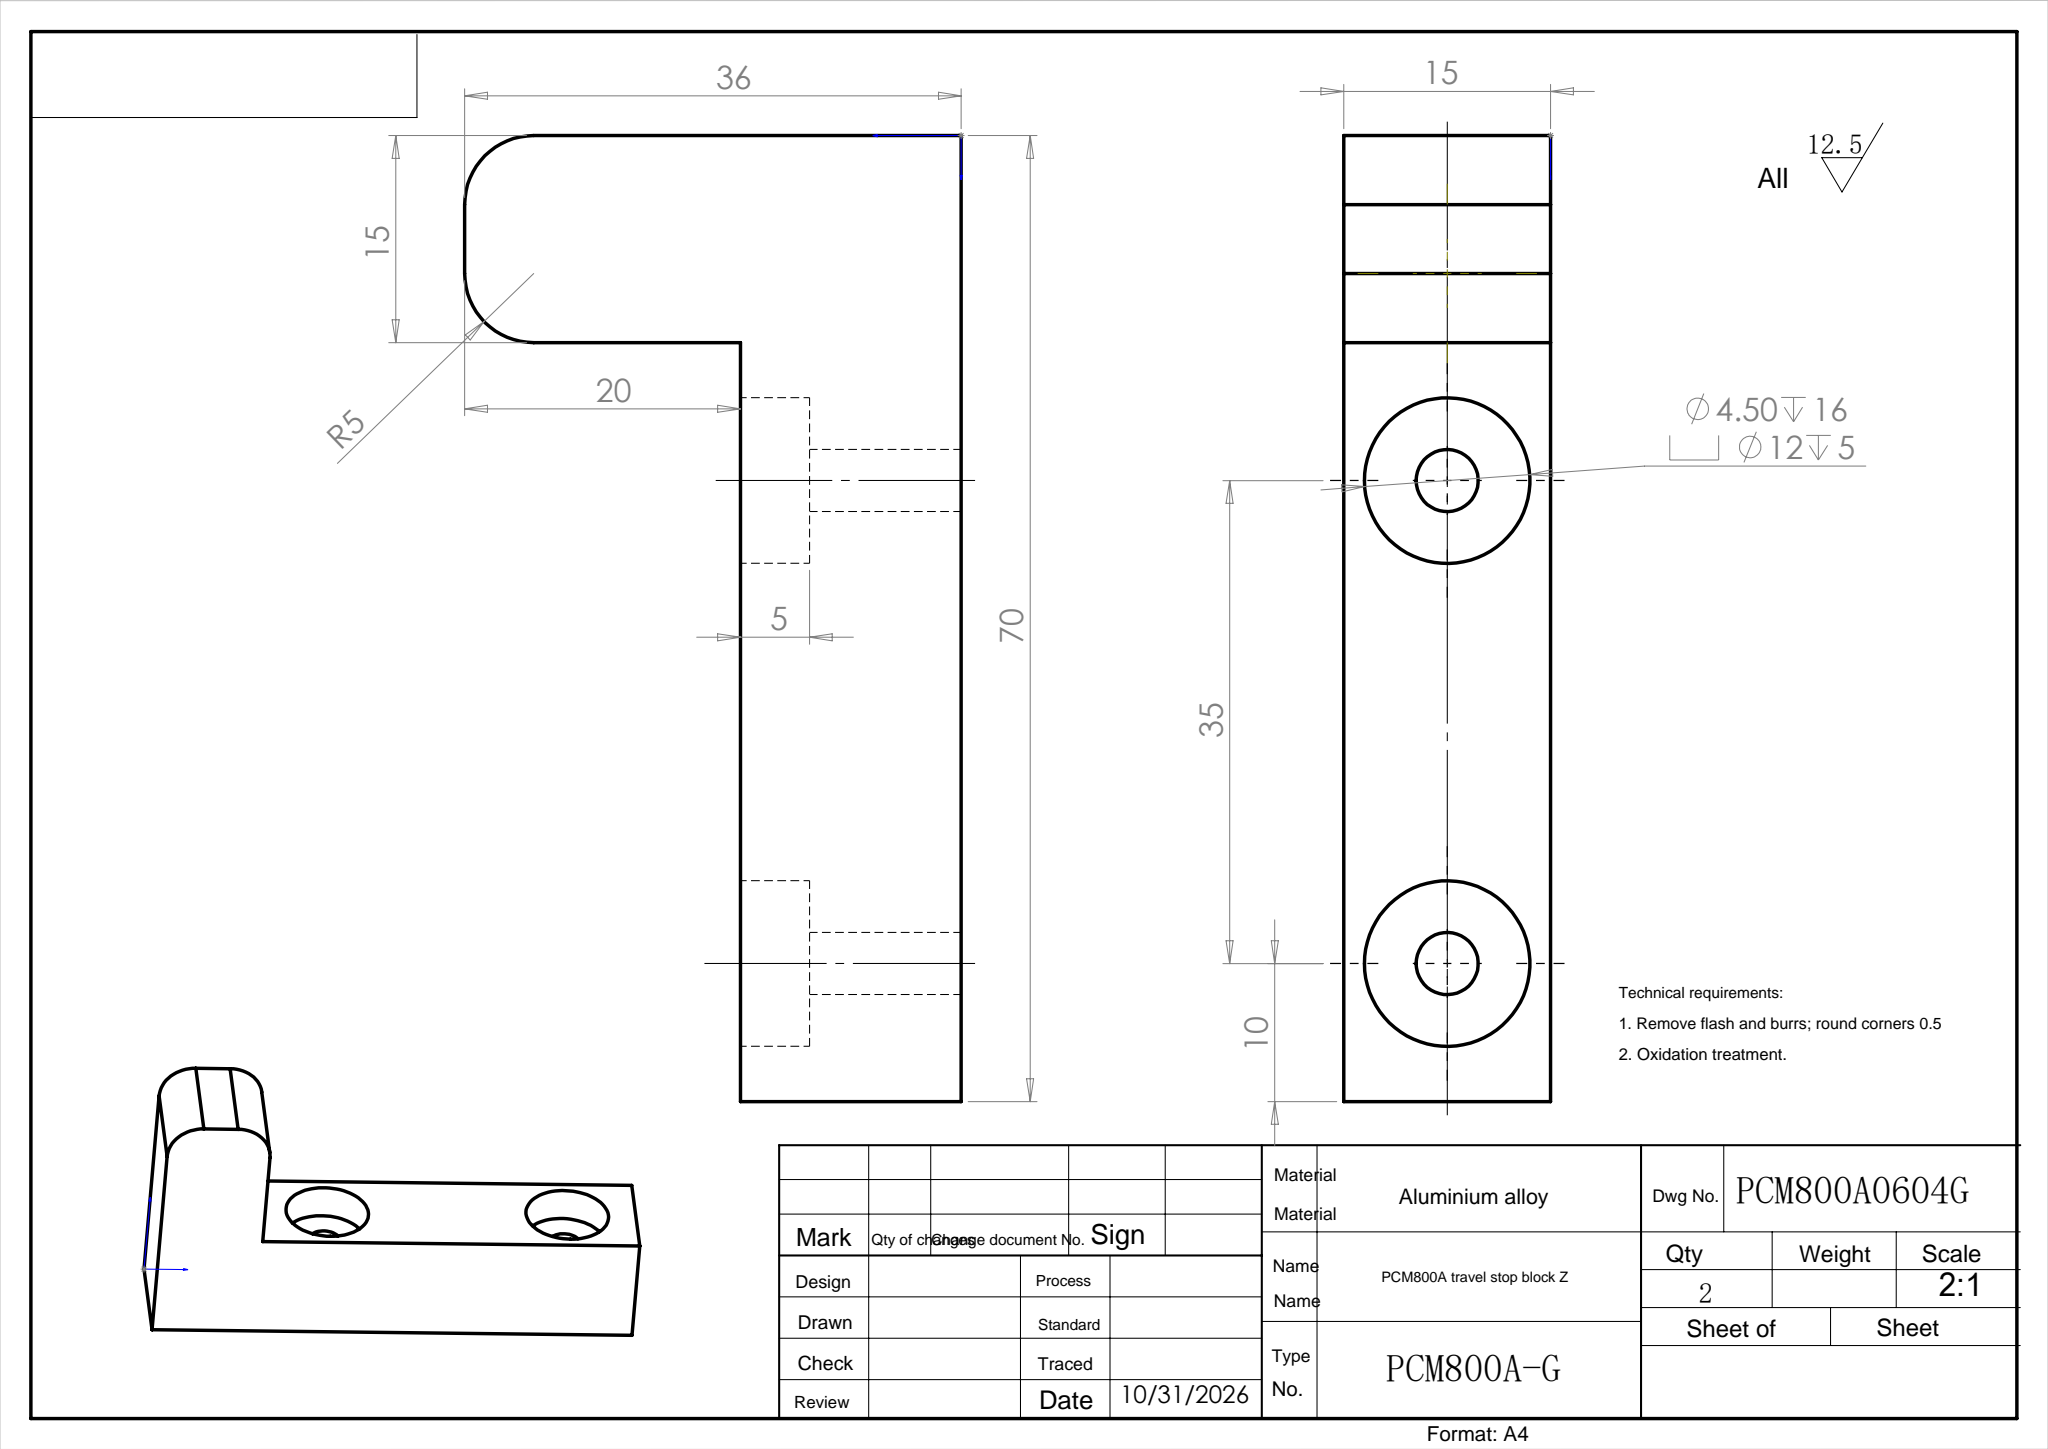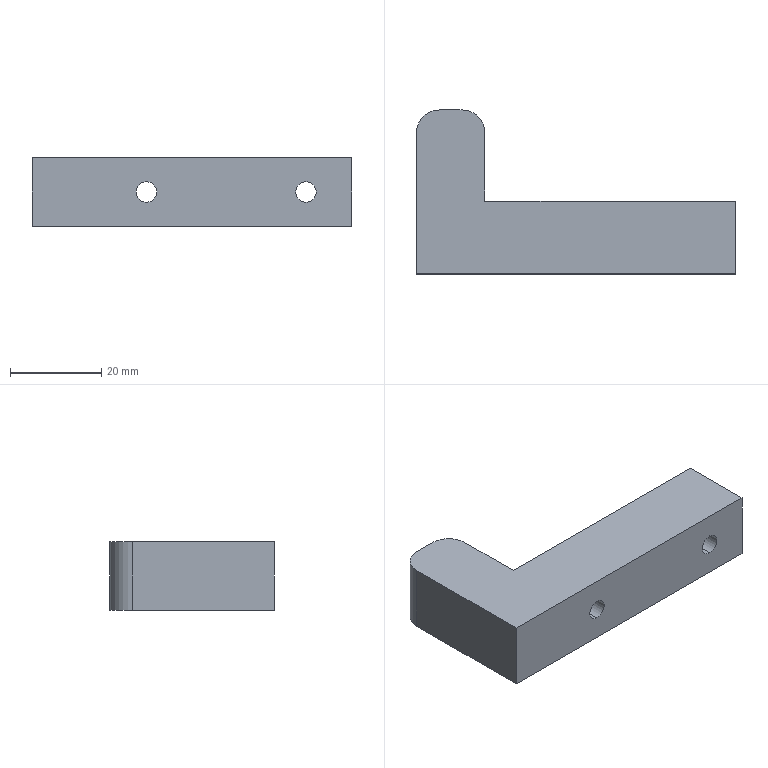Part | SolidWorks | features Extrusion 1, Fillet 1, HoleWzd 1 | 1 solid | 20 faces | box 70 x 36 x 15 mm | volume 19658 mm3 | cylinder 10 | plane 10 | commonest cylinder face diameters 4.5 x4 12 x4 10 x2
STEP:
#1=CARTESIAN_POINT('',(25.,11.,1.5));
#2=VERTEX_POINT('',#1);
#3=CARTESIAN_POINT('',(25.,11.,13.5));
#4=VERTEX_POINT('',#3);
#5=CARTESIAN_POINT('',(25.,11.,7.5));
#6=DIRECTION('',(0.,1.,0.));
#7=DIRECTION('',(0.,0.,1.));
#8=AXIS2_PLACEMENT_3D('',#5,#6,#7);
#9=CIRCLE('',#8,6.);
#10=EDGE_CURVE('',#2,#4,#9,.T.);
#11=ORIENTED_EDGE('',*,*,#10,.F.);
#12=CARTESIAN_POINT('',(25.,16.,1.5));
#13=VERTEX_POINT('',#12);
#14=CARTESIAN_POINT('',(25.,16.,1.5));
#15=DIRECTION('',(0.,1.,0.));
#16=VECTOR('',#15,1000.);
#17=LINE('',#14,#16);
#18=EDGE_CURVE('',#2,#13,#17,.T.);
#19=ORIENTED_EDGE('',*,*,#18,.T.);
#20=CARTESIAN_POINT('',(25.,16.,13.5));
#21=VERTEX_POINT('',#20);
#22=CARTESIAN_POINT('',(25.,16.,7.5));
#23=DIRECTION('',(0.,1.,0.));
#24=DIRECTION('',(0.,0.,1.));
#25=AXIS2_PLACEMENT_3D('',#22,#23,#24);
#26=CIRCLE('',#25,6.);
#27=EDGE_CURVE('',#13,#21,#26,.T.);
#28=ORIENTED_EDGE('',*,*,#27,.T.);
#29=CARTESIAN_POINT('',(25.,16.,13.5));
#30=DIRECTION('',(0.,1.,0.));
#31=VECTOR('',#30,1000.);
#32=LINE('',#29,#31);
#33=EDGE_CURVE('',#4,#21,#32,.T.);
#34=ORIENTED_EDGE('',*,*,#33,.F.);
#35=EDGE_LOOP('',(#11,#19,#28,#34));
#36=FACE_OUTER_BOUND('',#35,.T.);
#37=CARTESIAN_POINT('',(25.,16.,7.5));
#38=DIRECTION('',(0.,1.,0.));
#39=DIRECTION('',(0.,0.,1.));
#40=AXIS2_PLACEMENT_3D('',#37,#38,#39);
#41=CYLINDRICAL_SURFACE('',#40,6.);
#42=ADVANCED_FACE('',(#36),#41,.F.);
#43=CARTESIAN_POINT('',(25.,0.,5.25));
#44=VERTEX_POINT('',#43);
#45=CARTESIAN_POINT('',(25.,0.,9.75));
#46=VERTEX_POINT('',#45);
#47=CARTESIAN_POINT('',(25.,0.,7.5));
#48=DIRECTION('',(0.,1.,0.));
#49=DIRECTION('',(0.,0.,1.));
#50=AXIS2_PLACEMENT_3D('',#47,#48,#49);
#51=CIRCLE('',#50,2.25);
#52=EDGE_CURVE('',#44,#46,#51,.T.);
#53=ORIENTED_EDGE('',*,*,#52,.F.);
#54=CARTESIAN_POINT('',(25.,11.,5.25));
#55=VERTEX_POINT('',#54);
#56=CARTESIAN_POINT('',(25.,16.,5.25));
#57=DIRECTION('',(0.,1.,0.));
#58=VECTOR('',#57,1000.);
#59=LINE('',#56,#58);
#60=EDGE_CURVE('',#44,#55,#59,.T.);
#61=ORIENTED_EDGE('',*,*,#60,.T.);
#62=CARTESIAN_POINT('',(25.,11.,9.75));
#63=VERTEX_POINT('',#62);
#64=CARTESIAN_POINT('',(25.,11.,7.5));
#65=DIRECTION('',(0.,1.,0.));
#66=DIRECTION('',(0.,0.,1.));
#67=AXIS2_PLACEMENT_3D('',#64,#65,#66);
#68=CIRCLE('',#67,2.25);
#69=EDGE_CURVE('',#55,#63,#68,.T.);
#70=ORIENTED_EDGE('',*,*,#69,.T.);
#71=CARTESIAN_POINT('',(25.,16.,9.75));
#72=DIRECTION('',(0.,1.,0.));
#73=VECTOR('',#72,1000.);
#74=LINE('',#71,#73);
#75=EDGE_CURVE('',#46,#63,#74,.T.);
#76=ORIENTED_EDGE('',*,*,#75,.F.);
#77=EDGE_LOOP('',(#53,#61,#70,#76));
#78=FACE_OUTER_BOUND('',#77,.T.);
#79=CARTESIAN_POINT('',(25.,16.,7.5));
#80=DIRECTION('',(0.,1.,0.));
#81=DIRECTION('',(0.,0.,1.));
#82=AXIS2_PLACEMENT_3D('',#79,#80,#81);
#83=CYLINDRICAL_SURFACE('',#82,2.25);
#84=ADVANCED_FACE('',(#78),#83,.F.);
#85=CARTESIAN_POINT('',(60.,11.,1.5));
#86=VERTEX_POINT('',#85);
#87=CARTESIAN_POINT('',(60.,11.,13.5));
#88=VERTEX_POINT('',#87);
#89=CARTESIAN_POINT('',(60.,11.,7.5));
#90=DIRECTION('',(0.,1.,0.));
#91=DIRECTION('',(0.,0.,1.));
#92=AXIS2_PLACEMENT_3D('',#89,#90,#91);
#93=CIRCLE('',#92,6.);
#94=EDGE_CURVE('',#86,#88,#93,.T.);
#95=ORIENTED_EDGE('',*,*,#94,.F.);
#96=CARTESIAN_POINT('',(60.,16.,1.5));
#97=VERTEX_POINT('',#96);
#98=CARTESIAN_POINT('',(60.,16.,1.5));
#99=DIRECTION('',(0.,1.,0.));
#100=VECTOR('',#99,1000.);
#101=LINE('',#98,#100);
#102=EDGE_CURVE('',#86,#97,#101,.T.);
#103=ORIENTED_EDGE('',*,*,#102,.T.);
#104=CARTESIAN_POINT('',(60.,16.,13.5));
#105=VERTEX_POINT('',#104);
#106=CARTESIAN_POINT('',(60.,16.,7.5));
#107=DIRECTION('',(0.,1.,0.));
#108=DIRECTION('',(0.,0.,1.));
#109=AXIS2_PLACEMENT_3D('',#106,#107,#108);
#110=CIRCLE('',#109,6.);
#111=EDGE_CURVE('',#97,#105,#110,.T.);
#112=ORIENTED_EDGE('',*,*,#111,.T.);
#113=CARTESIAN_POINT('',(60.,16.,13.5));
#114=DIRECTION('',(0.,1.,0.));
#115=VECTOR('',#114,1000.);
#116=LINE('',#113,#115);
#117=EDGE_CURVE('',#88,#105,#116,.T.);
#118=ORIENTED_EDGE('',*,*,#117,.F.);
#119=EDGE_LOOP('',(#95,#103,#112,#118));
#120=FACE_OUTER_BOUND('',#119,.T.);
#121=CARTESIAN_POINT('',(60.,16.,7.5));
#122=DIRECTION('',(0.,1.,0.));
#123=DIRECTION('',(0.,0.,1.));
#124=AXIS2_PLACEMENT_3D('',#121,#122,#123);
#125=CYLINDRICAL_SURFACE('',#124,6.);
#126=ADVANCED_FACE('',(#120),#125,.F.);
#127=CARTESIAN_POINT('',(60.,0.,5.25));
#128=VERTEX_POINT('',#127);
#129=CARTESIAN_POINT('',(60.,0.,9.75));
#130=VERTEX_POINT('',#129);
#131=CARTESIAN_POINT('',(60.,0.,7.5));
#132=DIRECTION('',(0.,1.,0.));
#133=DIRECTION('',(0.,0.,1.));
#134=AXIS2_PLACEMENT_3D('',#131,#132,#133);
#135=CIRCLE('',#134,2.25);
#136=EDGE_CURVE('',#128,#130,#135,.T.);
#137=ORIENTED_EDGE('',*,*,#136,.F.);
#138=CARTESIAN_POINT('',(60.,11.,5.25));
#139=VERTEX_POINT('',#138);
#140=CARTESIAN_POINT('',(60.,16.,5.25));
#141=DIRECTION('',(0.,1.,0.));
#142=VECTOR('',#141,1000.);
#143=LINE('',#140,#142);
#144=EDGE_CURVE('',#128,#139,#143,.T.);
#145=ORIENTED_EDGE('',*,*,#144,.T.);
#146=CARTESIAN_POINT('',(60.,11.,9.75));
#147=VERTEX_POINT('',#146);
#148=CARTESIAN_POINT('',(60.,11.,7.5));
#149=DIRECTION('',(0.,1.,0.));
#150=DIRECTION('',(0.,0.,1.));
#151=AXIS2_PLACEMENT_3D('',#148,#149,#150);
#152=CIRCLE('',#151,2.25);
#153=EDGE_CURVE('',#139,#147,#152,.T.);
#154=ORIENTED_EDGE('',*,*,#153,.T.);
#155=CARTESIAN_POINT('',(60.,16.,9.75));
#156=DIRECTION('',(0.,1.,0.));
#157=VECTOR('',#156,1000.);
#158=LINE('',#155,#157);
#159=EDGE_CURVE('',#130,#147,#158,.T.);
#160=ORIENTED_EDGE('',*,*,#159,.F.);
#161=EDGE_LOOP('',(#137,#145,#154,#160));
#162=FACE_OUTER_BOUND('',#161,.T.);
#163=CARTESIAN_POINT('',(60.,16.,7.5));
#164=DIRECTION('',(0.,1.,0.));
#165=DIRECTION('',(0.,0.,1.));
#166=AXIS2_PLACEMENT_3D('',#163,#164,#165);
#167=CYLINDRICAL_SURFACE('',#166,2.25);
#168=ADVANCED_FACE('',(#162),#167,.F.);
#169=CARTESIAN_POINT('',(25.,0.,7.5));
#170=DIRECTION('',(0.,1.,0.));
#171=DIRECTION('',(0.,0.,1.));
#172=AXIS2_PLACEMENT_3D('',#169,#170,#171);
#173=CIRCLE('',#172,2.25);
#174=EDGE_CURVE('',#46,#44,#173,.T.);
#175=ORIENTED_EDGE('',*,*,#174,.T.);
#176=ORIENTED_EDGE('',*,*,#52,.T.);
#177=EDGE_LOOP('',(#175,#176));
#178=FACE_BOUND('',#177,.T.);
#179=CARTESIAN_POINT('',(60.,0.,7.5));
#180=DIRECTION('',(0.,1.,0.));
#181=DIRECTION('',(0.,0.,1.));
#182=AXIS2_PLACEMENT_3D('',#179,#180,#181);
#183=CIRCLE('',#182,2.25);
#184=EDGE_CURVE('',#130,#128,#183,.T.);
#185=ORIENTED_EDGE('',*,*,#184,.T.);
#186=ORIENTED_EDGE('',*,*,#136,.T.);
#187=EDGE_LOOP('',(#185,#186));
#188=FACE_BOUND('',#187,.T.);
#189=CARTESIAN_POINT('',(0.,0.,0.));
#190=VERTEX_POINT('',#189);
#191=CARTESIAN_POINT('',(70.,0.,0.));
#192=VERTEX_POINT('',#191);
#193=CARTESIAN_POINT('',(0.,0.,0.));
#194=DIRECTION('',(1.,0.,0.));
#195=VECTOR('',#194,1000.);
#196=LINE('',#193,#195);
#197=EDGE_CURVE('',#190,#192,#196,.T.);
#198=ORIENTED_EDGE('',*,*,#197,.T.);
#199=CARTESIAN_POINT('',(70.,0.,15.));
#200=VERTEX_POINT('',#199);
#201=CARTESIAN_POINT('',(70.,0.,15.));
#202=DIRECTION('',(0.,0.,-1.));
#203=VECTOR('',#202,1000.);
#204=LINE('',#201,#203);
#205=EDGE_CURVE('',#200,#192,#204,.T.);
#206=ORIENTED_EDGE('',*,*,#205,.F.);
#207=CARTESIAN_POINT('',(0.,0.,15.));
#208=VERTEX_POINT('',#207);
#209=CARTESIAN_POINT('',(0.,0.,15.));
#210=DIRECTION('',(1.,0.,0.));
#211=VECTOR('',#210,1000.);
#212=LINE('',#209,#211);
#213=EDGE_CURVE('',#208,#200,#212,.T.);
#214=ORIENTED_EDGE('',*,*,#213,.F.);
#215=CARTESIAN_POINT('',(0.,0.,15.));
#216=DIRECTION('',(0.,0.,-1.));
#217=VECTOR('',#216,1000.);
#218=LINE('',#215,#217);
#219=EDGE_CURVE('',#208,#190,#218,.T.);
#220=ORIENTED_EDGE('',*,*,#219,.T.);
#221=EDGE_LOOP('',(#198,#206,#214,#220));
#222=FACE_OUTER_BOUND('',#221,.T.);
#223=CARTESIAN_POINT('',(0.,0.,15.));
#224=DIRECTION('',(0.,1.,0.));
#225=DIRECTION('',(0.,0.,1.));
#226=AXIS2_PLACEMENT_3D('',#223,#224,#225);
#227=PLANE('',#226);
#228=ADVANCED_FACE('',(#178,#188,#222),#227,.F.);
#229=CARTESIAN_POINT('',(70.,16.,0.));
#230=VERTEX_POINT('',#229);
#231=CARTESIAN_POINT('',(70.,0.,0.));
#232=DIRECTION('',(0.,1.,0.));
#233=VECTOR('',#232,1000.);
#234=LINE('',#231,#233);
#235=EDGE_CURVE('',#192,#230,#234,.T.);
#236=ORIENTED_EDGE('',*,*,#235,.T.);
#237=CARTESIAN_POINT('',(70.,16.,15.));
#238=VERTEX_POINT('',#237);
#239=CARTESIAN_POINT('',(70.,16.,15.));
#240=DIRECTION('',(0.,0.,-1.));
#241=VECTOR('',#240,1000.);
#242=LINE('',#239,#241);
#243=EDGE_CURVE('',#238,#230,#242,.T.);
#244=ORIENTED_EDGE('',*,*,#243,.F.);
#245=CARTESIAN_POINT('',(70.,0.,15.));
#246=DIRECTION('',(0.,1.,0.));
#247=VECTOR('',#246,1000.);
#248=LINE('',#245,#247);
#249=EDGE_CURVE('',#200,#238,#248,.T.);
#250=ORIENTED_EDGE('',*,*,#249,.F.);
#251=ORIENTED_EDGE('',*,*,#205,.T.);
#252=EDGE_LOOP('',(#236,#244,#250,#251));
#253=FACE_OUTER_BOUND('',#252,.T.);
#254=CARTESIAN_POINT('',(70.,0.,15.));
#255=DIRECTION('',(-1.,0.,0.));
#256=DIRECTION('',(0.,0.,1.));
#257=AXIS2_PLACEMENT_3D('',#254,#255,#256);
#258=PLANE('',#257);
#259=ADVANCED_FACE('',(#253),#258,.F.);
#260=CARTESIAN_POINT('',(25.,16.,7.5));
#261=DIRECTION('',(0.,1.,0.));
#262=DIRECTION('',(0.,0.,1.));
#263=AXIS2_PLACEMENT_3D('',#260,#261,#262);
#264=CIRCLE('',#263,6.);
#265=EDGE_CURVE('',#21,#13,#264,.T.);
#266=ORIENTED_EDGE('',*,*,#265,.F.);
#267=ORIENTED_EDGE('',*,*,#27,.F.);
#268=EDGE_LOOP('',(#266,#267));
#269=FACE_BOUND('',#268,.T.);
#270=CARTESIAN_POINT('',(60.,16.,7.5));
#271=DIRECTION('',(0.,1.,0.));
#272=DIRECTION('',(0.,0.,1.));
#273=AXIS2_PLACEMENT_3D('',#270,#271,#272);
#274=CIRCLE('',#273,6.);
#275=EDGE_CURVE('',#105,#97,#274,.T.);
#276=ORIENTED_EDGE('',*,*,#275,.F.);
#277=ORIENTED_EDGE('',*,*,#111,.F.);
#278=EDGE_LOOP('',(#276,#277));
#279=FACE_BOUND('',#278,.T.);
#280=CARTESIAN_POINT('',(15.,16.,0.));
#281=VERTEX_POINT('',#280);
#282=CARTESIAN_POINT('',(70.,16.,0.));
#283=DIRECTION('',(-1.,0.,0.));
#284=VECTOR('',#283,1000.);
#285=LINE('',#282,#284);
#286=EDGE_CURVE('',#230,#281,#285,.T.);
#287=ORIENTED_EDGE('',*,*,#286,.T.);
#288=CARTESIAN_POINT('',(15.,16.,15.));
#289=VERTEX_POINT('',#288);
#290=CARTESIAN_POINT('',(15.,16.,15.));
#291=DIRECTION('',(0.,0.,-1.));
#292=VECTOR('',#291,1000.);
#293=LINE('',#290,#292);
#294=EDGE_CURVE('',#289,#281,#293,.T.);
#295=ORIENTED_EDGE('',*,*,#294,.F.);
#296=CARTESIAN_POINT('',(70.,16.,15.));
#297=DIRECTION('',(-1.,0.,0.));
#298=VECTOR('',#297,1000.);
#299=LINE('',#296,#298);
#300=EDGE_CURVE('',#238,#289,#299,.T.);
#301=ORIENTED_EDGE('',*,*,#300,.F.);
#302=ORIENTED_EDGE('',*,*,#243,.T.);
#303=EDGE_LOOP('',(#287,#295,#301,#302));
#304=FACE_OUTER_BOUND('',#303,.T.);
#305=CARTESIAN_POINT('',(70.,16.,15.));
#306=DIRECTION('',(0.,-1.,0.));
#307=DIRECTION('',(1.,0.,0.));
#308=AXIS2_PLACEMENT_3D('',#305,#306,#307);
#309=PLANE('',#308);
#310=ADVANCED_FACE('',(#269,#279,#304),#309,.F.);
#311=CARTESIAN_POINT('',(15.,31.,0.));
#312=VERTEX_POINT('',#311);
#313=CARTESIAN_POINT('',(15.,16.,0.));
#314=DIRECTION('',(0.,1.,0.));
#315=VECTOR('',#314,1000.);
#316=LINE('',#313,#315);
#317=EDGE_CURVE('',#281,#312,#316,.T.);
#318=ORIENTED_EDGE('',*,*,#317,.T.);
#319=CARTESIAN_POINT('',(15.,31.,15.));
#320=VERTEX_POINT('',#319);
#321=CARTESIAN_POINT('',(15.,31.,15.));
#322=DIRECTION('',(0.,0.,1.));
#323=VECTOR('',#322,1000.);
#324=LINE('',#321,#323);
#325=EDGE_CURVE('',#312,#320,#324,.T.);
#326=ORIENTED_EDGE('',*,*,#325,.T.);
#327=CARTESIAN_POINT('',(15.,16.,15.));
#328=DIRECTION('',(0.,1.,0.));
#329=VECTOR('',#328,1000.);
#330=LINE('',#327,#329);
#331=EDGE_CURVE('',#289,#320,#330,.T.);
#332=ORIENTED_EDGE('',*,*,#331,.F.);
#333=ORIENTED_EDGE('',*,*,#294,.T.);
#334=EDGE_LOOP('',(#318,#326,#332,#333));
#335=FACE_OUTER_BOUND('',#334,.T.);
#336=CARTESIAN_POINT('',(15.,16.,15.));
#337=DIRECTION('',(-1.,0.,0.));
#338=DIRECTION('',(0.,0.,1.));
#339=AXIS2_PLACEMENT_3D('',#336,#337,#338);
#340=PLANE('',#339);
#341=ADVANCED_FACE('',(#335),#340,.F.);
#342=CARTESIAN_POINT('',(10.,36.,0.));
#343=VERTEX_POINT('',#342);
#344=CARTESIAN_POINT('',(5.,36.,0.));
#345=VERTEX_POINT('',#344);
#346=CARTESIAN_POINT('',(15.,36.,0.));
#347=DIRECTION('',(-1.,0.,0.));
#348=VECTOR('',#347,1000.);
#349=LINE('',#346,#348);
#350=EDGE_CURVE('',#343,#345,#349,.T.);
#351=ORIENTED_EDGE('',*,*,#350,.T.);
#352=CARTESIAN_POINT('',(5.,36.,15.));
#353=VERTEX_POINT('',#352);
#354=CARTESIAN_POINT('',(5.,36.,15.));
#355=DIRECTION('',(0.,0.,1.));
#356=VECTOR('',#355,1000.);
#357=LINE('',#354,#356);
#358=EDGE_CURVE('',#345,#353,#357,.T.);
#359=ORIENTED_EDGE('',*,*,#358,.T.);
#360=CARTESIAN_POINT('',(10.,36.,15.));
#361=VERTEX_POINT('',#360);
#362=CARTESIAN_POINT('',(15.,36.,15.));
#363=DIRECTION('',(-1.,0.,0.));
#364=VECTOR('',#363,1000.);
#365=LINE('',#362,#364);
#366=EDGE_CURVE('',#361,#353,#365,.T.);
#367=ORIENTED_EDGE('',*,*,#366,.F.);
#368=CARTESIAN_POINT('',(10.,36.,15.));
#369=DIRECTION('',(0.,0.,-1.));
#370=VECTOR('',#369,1000.);
#371=LINE('',#368,#370);
#372=EDGE_CURVE('',#361,#343,#371,.T.);
#373=ORIENTED_EDGE('',*,*,#372,.T.);
#374=EDGE_LOOP('',(#351,#359,#367,#373));
#375=FACE_OUTER_BOUND('',#374,.T.);
#376=CARTESIAN_POINT('',(15.,36.,15.));
#377=DIRECTION('',(0.,-1.,0.));
#378=DIRECTION('',(0.,0.,-1.));
#379=AXIS2_PLACEMENT_3D('',#376,#377,#378);
#380=PLANE('',#379);
#381=ADVANCED_FACE('',(#375),#380,.F.);
#382=CARTESIAN_POINT('',(0.,31.,15.));
#383=VERTEX_POINT('',#382);
#384=CARTESIAN_POINT('',(0.,16.,15.));
#385=DIRECTION('',(0.,-1.,0.));
#386=VECTOR('',#385,1000.);
#387=LINE('',#384,#386);
#388=EDGE_CURVE('',#383,#208,#387,.T.);
#389=ORIENTED_EDGE('',*,*,#388,.F.);
#390=CARTESIAN_POINT('',(0.,31.,0.));
#391=VERTEX_POINT('',#390);
#392=CARTESIAN_POINT('',(0.,31.,15.));
#393=DIRECTION('',(0.,0.,-1.));
#394=VECTOR('',#393,1000.);
#395=LINE('',#392,#394);
#396=EDGE_CURVE('',#383,#391,#395,.T.);
#397=ORIENTED_EDGE('',*,*,#396,.T.);
#398=CARTESIAN_POINT('',(0.,36.,0.));
#399=DIRECTION('',(0.,-1.,0.));
#400=VECTOR('',#399,1000.);
#401=LINE('',#398,#400);
#402=EDGE_CURVE('',#391,#190,#401,.T.);
#403=ORIENTED_EDGE('',*,*,#402,.T.);
#404=ORIENTED_EDGE('',*,*,#219,.F.);
#405=EDGE_LOOP('',(#389,#397,#403,#404));
#406=FACE_OUTER_BOUND('',#405,.T.);
#407=CARTESIAN_POINT('',(0.,36.,15.));
#408=DIRECTION('',(1.,0.,0.));
#409=DIRECTION('',(0.,1.,0.));
#410=AXIS2_PLACEMENT_3D('',#407,#408,#409);
#411=PLANE('',#410);
#412=ADVANCED_FACE('',(#406),#411,.F.);
#413=ORIENTED_EDGE('',*,*,#366,.T.);
#414=CARTESIAN_POINT('',(5.,31.,15.));
#415=DIRECTION('',(0.,0.,1.));
#416=DIRECTION('',(1.,0.,0.));
#417=AXIS2_PLACEMENT_3D('',#414,#415,#416);
#418=CIRCLE('',#417,5.);
#419=EDGE_CURVE('',#353,#383,#418,.T.);
#420=ORIENTED_EDGE('',*,*,#419,.T.);
#421=ORIENTED_EDGE('',*,*,#388,.T.);
#422=ORIENTED_EDGE('',*,*,#213,.T.);
#423=ORIENTED_EDGE('',*,*,#249,.T.);
#424=ORIENTED_EDGE('',*,*,#300,.T.);
#425=ORIENTED_EDGE('',*,*,#331,.T.);
#426=CARTESIAN_POINT('',(10.,31.,15.));
#427=DIRECTION('',(0.,0.,1.));
#428=DIRECTION('',(1.,0.,0.));
#429=AXIS2_PLACEMENT_3D('',#426,#427,#428);
#430=CIRCLE('',#429,5.);
#431=EDGE_CURVE('',#320,#361,#430,.T.);
#432=ORIENTED_EDGE('',*,*,#431,.T.);
#433=EDGE_LOOP('',(#413,#420,#421,#422,#423,#424,#425,#432));
#434=FACE_OUTER_BOUND('',#433,.T.);
#435=CARTESIAN_POINT('',(0.,0.,15.));
#436=DIRECTION('',(0.,0.,1.));
#437=DIRECTION('',(1.,0.,0.));
#438=AXIS2_PLACEMENT_3D('',#435,#436,#437);
#439=PLANE('',#438);
#440=ADVANCED_FACE('',(#434),#439,.T.);
#441=ORIENTED_EDGE('',*,*,#402,.F.);
#442=CARTESIAN_POINT('',(5.,31.,0.));
#443=DIRECTION('',(0.,0.,-1.));
#444=DIRECTION('',(1.,0.,0.));
#445=AXIS2_PLACEMENT_3D('',#442,#443,#444);
#446=CIRCLE('',#445,5.);
#447=EDGE_CURVE('',#391,#345,#446,.T.);
#448=ORIENTED_EDGE('',*,*,#447,.T.);
#449=ORIENTED_EDGE('',*,*,#350,.F.);
#450=CARTESIAN_POINT('',(10.,31.,0.));
#451=DIRECTION('',(0.,0.,-1.));
#452=DIRECTION('',(1.,0.,0.));
#453=AXIS2_PLACEMENT_3D('',#450,#451,#452);
#454=CIRCLE('',#453,5.);
#455=EDGE_CURVE('',#343,#312,#454,.T.);
#456=ORIENTED_EDGE('',*,*,#455,.T.);
#457=ORIENTED_EDGE('',*,*,#317,.F.);
#458=ORIENTED_EDGE('',*,*,#286,.F.);
#459=ORIENTED_EDGE('',*,*,#235,.F.);
#460=ORIENTED_EDGE('',*,*,#197,.F.);
#461=EDGE_LOOP('',(#441,#448,#449,#456,#457,#458,#459,#460));
#462=FACE_OUTER_BOUND('',#461,.T.);
#463=CARTESIAN_POINT('',(0.,0.,0.));
#464=DIRECTION('',(0.,0.,1.));
#465=DIRECTION('',(1.,0.,0.));
#466=AXIS2_PLACEMENT_3D('',#463,#464,#465);
#467=PLANE('',#466);
#468=ADVANCED_FACE('',(#462),#467,.F.);
#469=ORIENTED_EDGE('',*,*,#419,.F.);
#470=ORIENTED_EDGE('',*,*,#358,.F.);
#471=ORIENTED_EDGE('',*,*,#447,.F.);
#472=ORIENTED_EDGE('',*,*,#396,.F.);
#473=EDGE_LOOP('',(#469,#470,#471,#472));
#474=FACE_OUTER_BOUND('',#473,.T.);
#475=CARTESIAN_POINT('',(5.,31.,15.));
#476=DIRECTION('',(0.,0.,-1.));
#477=DIRECTION('',(-1.,0.,0.));
#478=AXIS2_PLACEMENT_3D('',#475,#476,#477);
#479=CYLINDRICAL_SURFACE('',#478,5.);
#480=ADVANCED_FACE('',(#474),#479,.T.);
#481=ORIENTED_EDGE('',*,*,#431,.F.);
#482=ORIENTED_EDGE('',*,*,#325,.F.);
#483=ORIENTED_EDGE('',*,*,#455,.F.);
#484=ORIENTED_EDGE('',*,*,#372,.F.);
#485=EDGE_LOOP('',(#481,#482,#483,#484));
#486=FACE_OUTER_BOUND('',#485,.T.);
#487=CARTESIAN_POINT('',(10.,31.,15.));
#488=DIRECTION('',(0.,0.,-1.));
#489=DIRECTION('',(-1.,0.,0.));
#490=AXIS2_PLACEMENT_3D('',#487,#488,#489);
#491=CYLINDRICAL_SURFACE('',#490,5.);
#492=ADVANCED_FACE('',(#486),#491,.T.);
#493=ORIENTED_EDGE('',*,*,#144,.F.);
#494=ORIENTED_EDGE('',*,*,#184,.F.);
#495=ORIENTED_EDGE('',*,*,#159,.T.);
#496=CARTESIAN_POINT('',(60.,11.,7.5));
#497=DIRECTION('',(0.,1.,0.));
#498=DIRECTION('',(0.,0.,1.));
#499=AXIS2_PLACEMENT_3D('',#496,#497,#498);
#500=CIRCLE('',#499,2.25);
#501=EDGE_CURVE('',#147,#139,#500,.T.);
#502=ORIENTED_EDGE('',*,*,#501,.T.);
#503=EDGE_LOOP('',(#493,#494,#495,#502));
#504=FACE_OUTER_BOUND('',#503,.T.);
#505=CARTESIAN_POINT('',(60.,16.,7.5));
#506=DIRECTION('',(0.,1.,0.));
#507=DIRECTION('',(0.,0.,1.));
#508=AXIS2_PLACEMENT_3D('',#505,#506,#507);
#509=CYLINDRICAL_SURFACE('',#508,2.25);
#510=ADVANCED_FACE('',(#504),#509,.F.);
#511=ORIENTED_EDGE('',*,*,#501,.F.);
#512=ORIENTED_EDGE('',*,*,#153,.F.);
#513=EDGE_LOOP('',(#511,#512));
#514=FACE_BOUND('',#513,.T.);
#515=CARTESIAN_POINT('',(60.,11.,7.5));
#516=DIRECTION('',(0.,1.,0.));
#517=DIRECTION('',(0.,0.,1.));
#518=AXIS2_PLACEMENT_3D('',#515,#516,#517);
#519=CIRCLE('',#518,6.);
#520=EDGE_CURVE('',#88,#86,#519,.T.);
#521=ORIENTED_EDGE('',*,*,#520,.T.);
#522=ORIENTED_EDGE('',*,*,#94,.T.);
#523=EDGE_LOOP('',(#521,#522));
#524=FACE_OUTER_BOUND('',#523,.T.);
#525=CARTESIAN_POINT('',(62.25,11.,7.5));
#526=DIRECTION('',(0.,-1.,0.));
#527=DIRECTION('',(0.,0.,-1.));
#528=AXIS2_PLACEMENT_3D('',#525,#526,#527);
#529=PLANE('',#528);
#530=ADVANCED_FACE('',(#514,#524),#529,.F.);
#531=ORIENTED_EDGE('',*,*,#102,.F.);
#532=ORIENTED_EDGE('',*,*,#520,.F.);
#533=ORIENTED_EDGE('',*,*,#117,.T.);
#534=ORIENTED_EDGE('',*,*,#275,.T.);
#535=EDGE_LOOP('',(#531,#532,#533,#534));
#536=FACE_OUTER_BOUND('',#535,.T.);
#537=CARTESIAN_POINT('',(60.,16.,7.5));
#538=DIRECTION('',(0.,1.,0.));
#539=DIRECTION('',(0.,0.,1.));
#540=AXIS2_PLACEMENT_3D('',#537,#538,#539);
#541=CYLINDRICAL_SURFACE('',#540,6.);
#542=ADVANCED_FACE('',(#536),#541,.F.);
#543=ORIENTED_EDGE('',*,*,#60,.F.);
#544=ORIENTED_EDGE('',*,*,#174,.F.);
#545=ORIENTED_EDGE('',*,*,#75,.T.);
#546=CARTESIAN_POINT('',(25.,11.,7.5));
#547=DIRECTION('',(0.,1.,0.));
#548=DIRECTION('',(0.,0.,1.));
#549=AXIS2_PLACEMENT_3D('',#546,#547,#548);
#550=CIRCLE('',#549,2.25);
#551=EDGE_CURVE('',#63,#55,#550,.T.);
#552=ORIENTED_EDGE('',*,*,#551,.T.);
#553=EDGE_LOOP('',(#543,#544,#545,#552));
#554=FACE_OUTER_BOUND('',#553,.T.);
#555=CARTESIAN_POINT('',(25.,16.,7.5));
#556=DIRECTION('',(0.,1.,0.));
#557=DIRECTION('',(0.,0.,1.));
#558=AXIS2_PLACEMENT_3D('',#555,#556,#557);
#559=CYLINDRICAL_SURFACE('',#558,2.25);
#560=ADVANCED_FACE('',(#554),#559,.F.);
#561=ORIENTED_EDGE('',*,*,#551,.F.);
#562=ORIENTED_EDGE('',*,*,#69,.F.);
#563=EDGE_LOOP('',(#561,#562));
#564=FACE_BOUND('',#563,.T.);
#565=CARTESIAN_POINT('',(25.,11.,7.5));
#566=DIRECTION('',(0.,1.,0.));
#567=DIRECTION('',(0.,0.,1.));
#568=AXIS2_PLACEMENT_3D('',#565,#566,#567);
#569=CIRCLE('',#568,6.);
#570=EDGE_CURVE('',#4,#2,#569,.T.);
#571=ORIENTED_EDGE('',*,*,#570,.T.);
#572=ORIENTED_EDGE('',*,*,#10,.T.);
#573=EDGE_LOOP('',(#571,#572));
#574=FACE_OUTER_BOUND('',#573,.T.);
#575=CARTESIAN_POINT('',(27.25,11.,7.5));
#576=DIRECTION('',(0.,-1.,0.));
#577=DIRECTION('',(0.,0.,-1.));
#578=AXIS2_PLACEMENT_3D('',#575,#576,#577);
#579=PLANE('',#578);
#580=ADVANCED_FACE('',(#564,#574),#579,.F.);
#581=ORIENTED_EDGE('',*,*,#18,.F.);
#582=ORIENTED_EDGE('',*,*,#570,.F.);
#583=ORIENTED_EDGE('',*,*,#33,.T.);
#584=ORIENTED_EDGE('',*,*,#265,.T.);
#585=EDGE_LOOP('',(#581,#582,#583,#584));
#586=FACE_OUTER_BOUND('',#585,.T.);
#587=CARTESIAN_POINT('',(25.,16.,7.5));
#588=DIRECTION('',(0.,1.,0.));
#589=DIRECTION('',(0.,0.,1.));
#590=AXIS2_PLACEMENT_3D('',#587,#588,#589);
#591=CYLINDRICAL_SURFACE('',#590,6.);
#592=ADVANCED_FACE('',(#586),#591,.F.);
#593=CLOSED_SHELL('',(#42,#84,#126,#168,#228,#259,#310,#341,#381,#412,#440,#468,#480,#492,#510,#530,#542,#560,#580,#592));
#594=MANIFOLD_SOLID_BREP('',#593);
#595=CARTESIAN_POINT('',(0.,0.,0.));
#596=DIRECTION('',(0.,0.,1.));
#597=DIRECTION('',(1.,0.,0.));
#598=AXIS2_PLACEMENT_3D('',#595,#596,#597);
#599=(LENGTH_UNIT()NAMED_UNIT(*)SI_UNIT(.MILLI.,.METRE.));
#600=UNCERTAINTY_MEASURE_WITH_UNIT(LENGTH_MEASURE(0.00001),#599,'','');
#601=(NAMED_UNIT(*)PLANE_ANGLE_UNIT()SI_UNIT($,.RADIAN.));
#602=(NAMED_UNIT(*)SI_UNIT($,.STERADIAN.)SOLID_ANGLE_UNIT());
#603=(GEOMETRIC_REPRESENTATION_CONTEXT(3)GLOBAL_UNCERTAINTY_ASSIGNED_CONTEXT((#600))GLOBAL_UNIT_ASSIGNED_CONTEXT((#599,#601,#602))REPRESENTATION_CONTEXT('',''));
#604=ADVANCED_BREP_SHAPE_REPRESENTATION('',(#594,#598),#603);